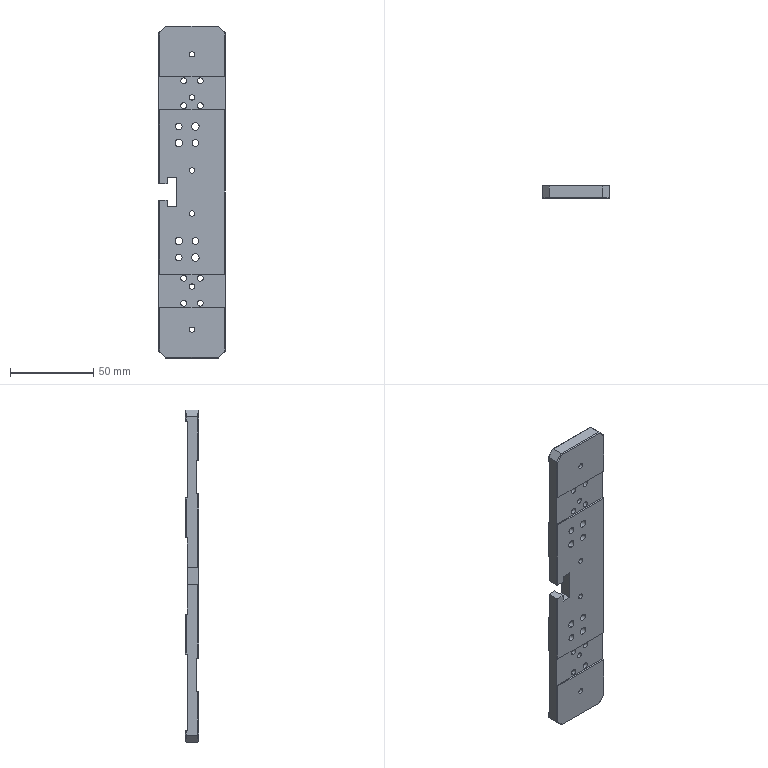Part | STEP file | A034 | 1 solid | 145 faces | box 40 x 8 x 200 mm | volume 52528 mm3 | plane 77 | cylinder 68 | commonest cylinder face diameters 3.5 x16 6.5 x16 3.242 x12 4 x8 4.5 x8 8 x8